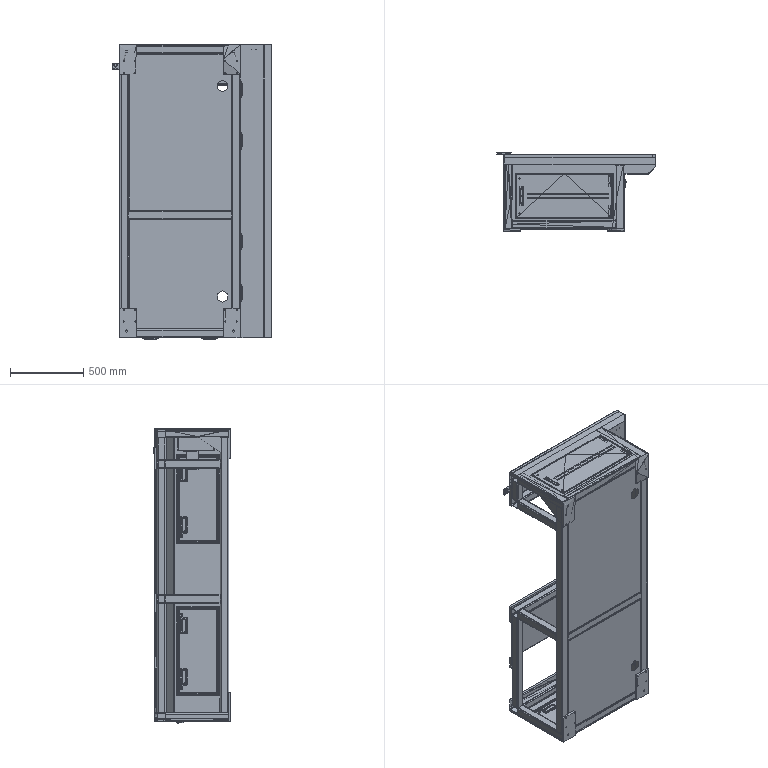Part | NX | features BREP 45 | 52 solids | 3170 faces | volume 11645432859295465956486677126374539909013734101819471668352754957128039835011836855041366573513841836032 mm3 | plane 1569 | cylinder 1220 | spline 156 | torus 130 | cone 95 | commonest cylinder face diameters 7 x143 4 x136 8 x132 6 x84 6.8 x77 16 x77